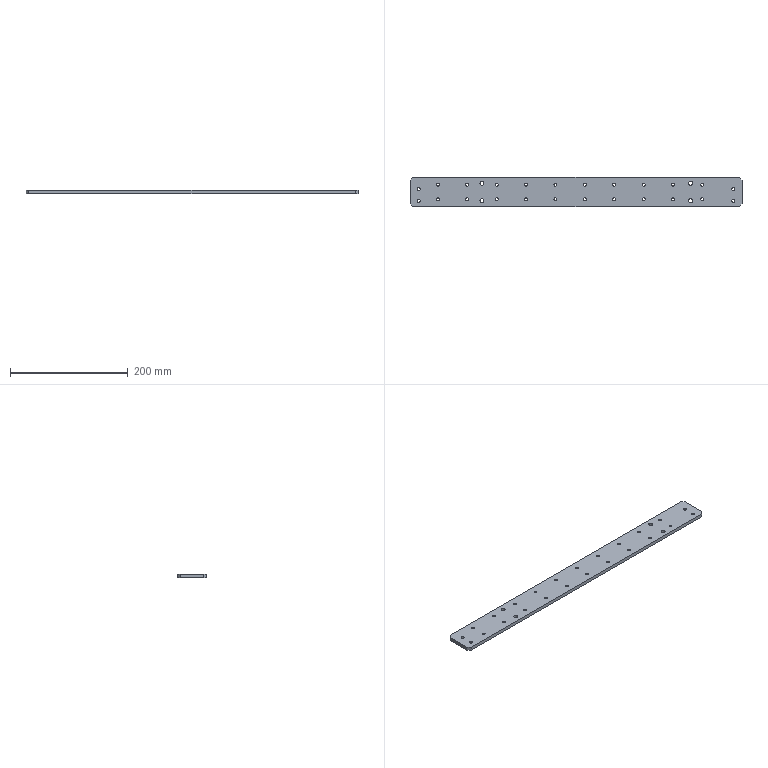Part | STEP file | J014-EBZ05-05-06 | 1 solid | 66 faces | box 565 x 50 x 6 mm | volume 165501 mm3 | cylinder 56 | plane 10 | commonest cylinder face diameters 5 x48 6.8 x8